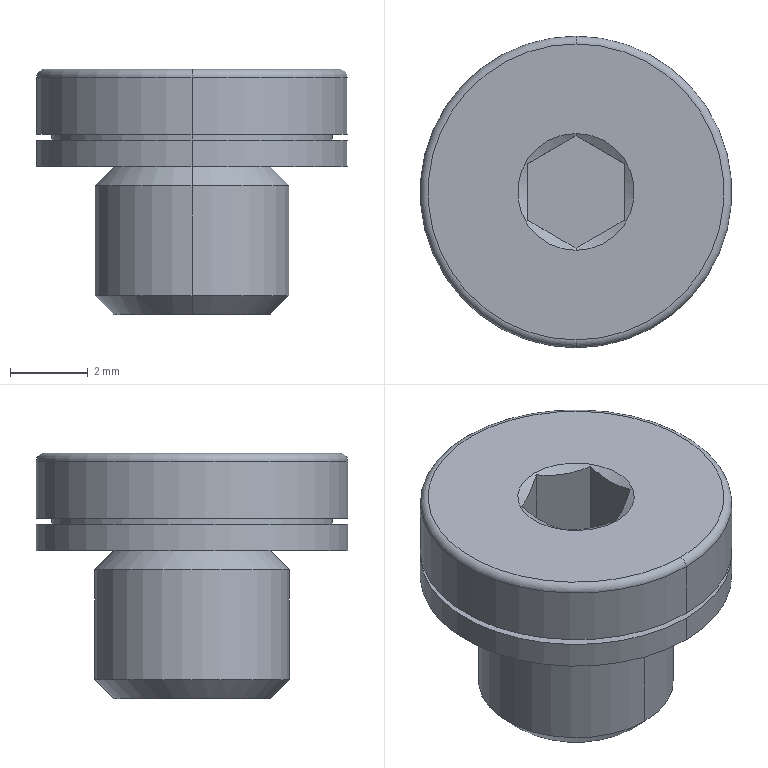Part | SolidWorks | features RefAxis 6, 3DProfileFeature 2, ICE 1, Revolution 1 | 1 solid | 28 faces | box 8 x 8 x 6.3 mm | volume 181.471 mm3 | plane 12 | cylinder 8 | cone 6 | torus 2 | commonest cylinder face diameters 8 x4 5 x2 7.2 x2
STEP:
#1=CARTESIAN_POINT('',(0.,-2.01,-3.8));
#2=VERTEX_POINT('',#1);
#3=CARTESIAN_POINT('',(0.,2.01,-3.8));
#4=VERTEX_POINT('',#3);
#5=CARTESIAN_POINT('',(0.,0.,-3.8));
#6=DIRECTION('',(0.,0.,1.));
#7=DIRECTION('',(0.,-1.,0.));
#8=AXIS2_PLACEMENT_3D('',#5,#6,#7);
#9=CIRCLE('',#8,2.01);
#10=EDGE_CURVE('',#2,#4,#9,.T.);
#11=ORIENTED_EDGE('',*,*,#10,.T.);
#12=CARTESIAN_POINT('',(0.,2.5,-3.309));
#13=VERTEX_POINT('',#12);
#14=CARTESIAN_POINT('',(0.,2.01,-3.8));
#15=DIRECTION('',(0.,0.7071,0.7071));
#16=VECTOR('',#15,1000.);
#17=LINE('',#14,#16);
#18=EDGE_CURVE('',#4,#13,#17,.T.);
#19=ORIENTED_EDGE('',*,*,#18,.T.);
#20=CARTESIAN_POINT('',(0.,-2.5,-3.309));
#21=VERTEX_POINT('',#20);
#22=CARTESIAN_POINT('',(0.,0.,-3.309));
#23=DIRECTION('',(0.,0.,1.));
#24=DIRECTION('',(0.,-1.,0.));
#25=AXIS2_PLACEMENT_3D('',#22,#23,#24);
#26=CIRCLE('',#25,2.5);
#27=EDGE_CURVE('',#21,#13,#26,.T.);
#28=ORIENTED_EDGE('',*,*,#27,.F.);
#29=CARTESIAN_POINT('',(0.,-2.01,-3.8));
#30=DIRECTION('',(0.,-0.7071,0.7071));
#31=VECTOR('',#30,1000.);
#32=LINE('',#29,#31);
#33=EDGE_CURVE('',#2,#21,#32,.T.);
#34=ORIENTED_EDGE('',*,*,#33,.F.);
#35=EDGE_LOOP('',(#11,#19,#28,#34));
#36=FACE_OUTER_BOUND('',#35,.T.);
#37=CARTESIAN_POINT('',(0.,0.,-3.8));
#38=DIRECTION('',(0.,0.,1.));
#39=DIRECTION('',(0.,-1.,0.));
#40=AXIS2_PLACEMENT_3D('',#37,#38,#39);
#41=CONICAL_SURFACE('',#40,2.01,0.7854);
#42=ADVANCED_FACE('',(#36),#41,.T.);
#43=ORIENTED_EDGE('',*,*,#27,.T.);
#44=CARTESIAN_POINT('',(0.,2.5,-0.4905));
#45=VERTEX_POINT('',#44);
#46=CARTESIAN_POINT('',(0.,2.5,-3.8));
#47=DIRECTION('',(0.,0.,1.));
#48=VECTOR('',#47,1000.);
#49=LINE('',#46,#48);
#50=EDGE_CURVE('',#13,#45,#49,.T.);
#51=ORIENTED_EDGE('',*,*,#50,.T.);
#52=CARTESIAN_POINT('',(0.,-2.5,-0.4905));
#53=VERTEX_POINT('',#52);
#54=CARTESIAN_POINT('',(0.,0.,-0.4905));
#55=DIRECTION('',(0.,0.,1.));
#56=DIRECTION('',(0.,-1.,0.));
#57=AXIS2_PLACEMENT_3D('',#54,#55,#56);
#58=CIRCLE('',#57,2.5);
#59=EDGE_CURVE('',#53,#45,#58,.T.);
#60=ORIENTED_EDGE('',*,*,#59,.F.);
#61=CARTESIAN_POINT('',(0.,-2.5,-3.8));
#62=DIRECTION('',(0.,0.,1.));
#63=VECTOR('',#62,1000.);
#64=LINE('',#61,#63);
#65=EDGE_CURVE('',#21,#53,#64,.T.);
#66=ORIENTED_EDGE('',*,*,#65,.F.);
#67=EDGE_LOOP('',(#43,#51,#60,#66));
#68=FACE_OUTER_BOUND('',#67,.T.);
#69=CARTESIAN_POINT('',(0.,0.,-3.8));
#70=DIRECTION('',(0.,0.,1.));
#71=DIRECTION('',(0.,-1.,0.));
#72=AXIS2_PLACEMENT_3D('',#69,#70,#71);
#73=CYLINDRICAL_SURFACE('',#72,2.5);
#74=ADVANCED_FACE('',(#68),#73,.T.);
#75=CARTESIAN_POINT('',(0.,-2.01,0.));
#76=VERTEX_POINT('',#75);
#77=CARTESIAN_POINT('',(0.,2.01,0.));
#78=VERTEX_POINT('',#77);
#79=CARTESIAN_POINT('',(0.,0.,0.));
#80=DIRECTION('',(0.,0.,1.));
#81=DIRECTION('',(0.,-1.,0.));
#82=AXIS2_PLACEMENT_3D('',#79,#80,#81);
#83=CIRCLE('',#82,2.01);
#84=EDGE_CURVE('',#76,#78,#83,.T.);
#85=ORIENTED_EDGE('',*,*,#84,.F.);
#86=CARTESIAN_POINT('',(0.,-2.5,-0.4905));
#87=DIRECTION('',(0.,-0.7071,-0.7071));
#88=VECTOR('',#87,1000.);
#89=LINE('',#86,#88);
#90=EDGE_CURVE('',#76,#53,#89,.T.);
#91=ORIENTED_EDGE('',*,*,#90,.T.);
#92=ORIENTED_EDGE('',*,*,#59,.T.);
#93=CARTESIAN_POINT('',(0.,2.5,-0.4905));
#94=DIRECTION('',(0.,0.7071,-0.7071));
#95=VECTOR('',#94,1000.);
#96=LINE('',#93,#95);
#97=EDGE_CURVE('',#78,#45,#96,.T.);
#98=ORIENTED_EDGE('',*,*,#97,.F.);
#99=EDGE_LOOP('',(#85,#91,#92,#98));
#100=FACE_OUTER_BOUND('',#99,.T.);
#101=CARTESIAN_POINT('',(0.,0.,-0.4905));
#102=DIRECTION('',(0.,0.,-1.));
#103=DIRECTION('',(0.,1.,0.));
#104=AXIS2_PLACEMENT_3D('',#101,#102,#103);
#105=CONICAL_SURFACE('',#104,2.5,0.7854);
#106=ADVANCED_FACE('',(#100),#105,.T.);
#107=CARTESIAN_POINT('',(0.,-4.,0.));
#108=VERTEX_POINT('',#107);
#109=CARTESIAN_POINT('',(0.,4.,0.));
#110=VERTEX_POINT('',#109);
#111=CARTESIAN_POINT('',(0.,0.,0.));
#112=DIRECTION('',(0.,0.,1.));
#113=DIRECTION('',(0.,-1.,0.));
#114=AXIS2_PLACEMENT_3D('',#111,#112,#113);
#115=CIRCLE('',#114,4.);
#116=EDGE_CURVE('',#108,#110,#115,.T.);
#117=ORIENTED_EDGE('',*,*,#116,.T.);
#118=CARTESIAN_POINT('',(0.,4.,0.6833));
#119=VERTEX_POINT('',#118);
#120=CARTESIAN_POINT('',(0.,4.,-3.8));
#121=DIRECTION('',(0.,0.,1.));
#122=VECTOR('',#121,1000.);
#123=LINE('',#120,#122);
#124=EDGE_CURVE('',#110,#119,#123,.T.);
#125=ORIENTED_EDGE('',*,*,#124,.T.);
#126=CARTESIAN_POINT('',(0.,-4.,0.6833));
#127=VERTEX_POINT('',#126);
#128=CARTESIAN_POINT('',(0.,0.,0.6833));
#129=DIRECTION('',(0.,0.,1.));
#130=DIRECTION('',(0.,-1.,0.));
#131=AXIS2_PLACEMENT_3D('',#128,#129,#130);
#132=CIRCLE('',#131,4.);
#133=EDGE_CURVE('',#127,#119,#132,.T.);
#134=ORIENTED_EDGE('',*,*,#133,.F.);
#135=CARTESIAN_POINT('',(0.,-4.,-3.8));
#136=DIRECTION('',(0.,0.,1.));
#137=VECTOR('',#136,1000.);
#138=LINE('',#135,#137);
#139=EDGE_CURVE('',#108,#127,#138,.T.);
#140=ORIENTED_EDGE('',*,*,#139,.F.);
#141=EDGE_LOOP('',(#117,#125,#134,#140));
#142=FACE_OUTER_BOUND('',#141,.T.);
#143=CARTESIAN_POINT('',(0.,0.,-3.8));
#144=DIRECTION('',(0.,0.,1.));
#145=DIRECTION('',(0.,-1.,0.));
#146=AXIS2_PLACEMENT_3D('',#143,#144,#145);
#147=CYLINDRICAL_SURFACE('',#146,4.);
#148=ADVANCED_FACE('',(#142),#147,.T.);
#149=CARTESIAN_POINT('',(0.,-3.6,0.6833));
#150=VERTEX_POINT('',#149);
#151=CARTESIAN_POINT('',(0.,3.6,0.6833));
#152=VERTEX_POINT('',#151);
#153=CARTESIAN_POINT('',(0.,0.,0.6833));
#154=DIRECTION('',(0.,0.,1.));
#155=DIRECTION('',(0.,-1.,0.));
#156=AXIS2_PLACEMENT_3D('',#153,#154,#155);
#157=CIRCLE('',#156,3.6);
#158=EDGE_CURVE('',#150,#152,#157,.T.);
#159=ORIENTED_EDGE('',*,*,#158,.T.);
#160=CARTESIAN_POINT('',(0.,3.6,0.8333));
#161=VERTEX_POINT('',#160);
#162=CARTESIAN_POINT('',(0.,3.6,-3.8));
#163=DIRECTION('',(0.,0.,1.));
#164=VECTOR('',#163,1000.);
#165=LINE('',#162,#164);
#166=EDGE_CURVE('',#152,#161,#165,.T.);
#167=ORIENTED_EDGE('',*,*,#166,.T.);
#168=CARTESIAN_POINT('',(0.,-3.6,0.8333));
#169=VERTEX_POINT('',#168);
#170=CARTESIAN_POINT('',(0.,0.,0.8333));
#171=DIRECTION('',(0.,0.,1.));
#172=DIRECTION('',(0.,-1.,0.));
#173=AXIS2_PLACEMENT_3D('',#170,#171,#172);
#174=CIRCLE('',#173,3.6);
#175=EDGE_CURVE('',#169,#161,#174,.T.);
#176=ORIENTED_EDGE('',*,*,#175,.F.);
#177=CARTESIAN_POINT('',(0.,-3.6,-3.8));
#178=DIRECTION('',(0.,0.,1.));
#179=VECTOR('',#178,1000.);
#180=LINE('',#177,#179);
#181=EDGE_CURVE('',#150,#169,#180,.T.);
#182=ORIENTED_EDGE('',*,*,#181,.F.);
#183=EDGE_LOOP('',(#159,#167,#176,#182));
#184=FACE_OUTER_BOUND('',#183,.T.);
#185=CARTESIAN_POINT('',(0.,0.,-3.8));
#186=DIRECTION('',(0.,0.,1.));
#187=DIRECTION('',(0.,-1.,0.));
#188=AXIS2_PLACEMENT_3D('',#185,#186,#187);
#189=CYLINDRICAL_SURFACE('',#188,3.6);
#190=ADVANCED_FACE('',(#184),#189,.T.);
#191=CARTESIAN_POINT('',(0.,-4.,0.8333));
#192=VERTEX_POINT('',#191);
#193=CARTESIAN_POINT('',(0.,4.,0.8333));
#194=VERTEX_POINT('',#193);
#195=CARTESIAN_POINT('',(0.,0.,0.8333));
#196=DIRECTION('',(0.,0.,1.));
#197=DIRECTION('',(0.,-1.,0.));
#198=AXIS2_PLACEMENT_3D('',#195,#196,#197);
#199=CIRCLE('',#198,4.);
#200=EDGE_CURVE('',#192,#194,#199,.T.);
#201=ORIENTED_EDGE('',*,*,#200,.T.);
#202=CARTESIAN_POINT('',(0.,4.,2.3));
#203=VERTEX_POINT('',#202);
#204=CARTESIAN_POINT('',(0.,4.,-3.8));
#205=DIRECTION('',(0.,0.,1.));
#206=VECTOR('',#205,1000.);
#207=LINE('',#204,#206);
#208=EDGE_CURVE('',#194,#203,#207,.T.);
#209=ORIENTED_EDGE('',*,*,#208,.T.);
#210=CARTESIAN_POINT('',(0.,-4.,2.3));
#211=VERTEX_POINT('',#210);
#212=CARTESIAN_POINT('',(0.,0.,2.3));
#213=DIRECTION('',(0.,0.,1.));
#214=DIRECTION('',(0.,-1.,0.));
#215=AXIS2_PLACEMENT_3D('',#212,#213,#214);
#216=CIRCLE('',#215,4.);
#217=EDGE_CURVE('',#211,#203,#216,.T.);
#218=ORIENTED_EDGE('',*,*,#217,.F.);
#219=CARTESIAN_POINT('',(0.,-4.,-3.8));
#220=DIRECTION('',(0.,0.,1.));
#221=VECTOR('',#220,1000.);
#222=LINE('',#219,#221);
#223=EDGE_CURVE('',#192,#211,#222,.T.);
#224=ORIENTED_EDGE('',*,*,#223,.F.);
#225=EDGE_LOOP('',(#201,#209,#218,#224));
#226=FACE_OUTER_BOUND('',#225,.T.);
#227=CARTESIAN_POINT('',(0.,0.,-3.8));
#228=DIRECTION('',(0.,0.,1.));
#229=DIRECTION('',(0.,-1.,0.));
#230=AXIS2_PLACEMENT_3D('',#227,#228,#229);
#231=CYLINDRICAL_SURFACE('',#230,4.);
#232=ADVANCED_FACE('',(#226),#231,.T.);
#233=ORIENTED_EDGE('',*,*,#217,.T.);
#234=CARTESIAN_POINT('',(0.,3.8,2.5));
#235=VERTEX_POINT('',#234);
#236=CARTESIAN_POINT('',(0.,3.8,2.3));
#237=DIRECTION('',(1.,0.,0.));
#238=DIRECTION('',(0.,1.,0.));
#239=AXIS2_PLACEMENT_3D('',#236,#237,#238);
#240=CIRCLE('',#239,0.2);
#241=EDGE_CURVE('',#203,#235,#240,.T.);
#242=ORIENTED_EDGE('',*,*,#241,.T.);
#243=CARTESIAN_POINT('',(0.,-3.8,2.5));
#244=VERTEX_POINT('',#243);
#245=CARTESIAN_POINT('',(0.,0.,2.5));
#246=DIRECTION('',(0.,0.,1.));
#247=DIRECTION('',(0.,-1.,0.));
#248=AXIS2_PLACEMENT_3D('',#245,#246,#247);
#249=CIRCLE('',#248,3.8);
#250=EDGE_CURVE('',#244,#235,#249,.T.);
#251=ORIENTED_EDGE('',*,*,#250,.F.);
#252=CARTESIAN_POINT('',(0.,-3.8,2.3));
#253=DIRECTION('',(-1.,0.,0.));
#254=DIRECTION('',(0.,0.,1.));
#255=AXIS2_PLACEMENT_3D('',#252,#253,#254);
#256=CIRCLE('',#255,0.2);
#257=EDGE_CURVE('',#211,#244,#256,.T.);
#258=ORIENTED_EDGE('',*,*,#257,.F.);
#259=EDGE_LOOP('',(#233,#242,#251,#258));
#260=FACE_OUTER_BOUND('',#259,.T.);
#261=CARTESIAN_POINT('',(0.,0.,2.3));
#262=DIRECTION('',(0.,0.,1.));
#263=DIRECTION('',(0.,-1.,0.));
#264=AXIS2_PLACEMENT_3D('',#261,#262,#263);
#265=TOROIDAL_SURFACE('',#264,3.8,0.2);
#266=ADVANCED_FACE('',(#260),#265,.T.);
#267=CARTESIAN_POINT('',(-1.25,0.7217,2.467));
#268=VERTEX_POINT('',#267);
#269=CARTESIAN_POINT('',(0.,1.443,2.467));
#270=VERTEX_POINT('',#269);
#271=CARTESIAN_POINT('',(-1.25,0.7217,2.467));
#272=CARTESIAN_POINT('',(-1.046,0.8395,2.399));
#273=CARTESIAN_POINT('',(-0.8387,0.9591,2.356));
#274=CARTESIAN_POINT('',(-0.4136,1.205,2.356));
#275=CARTESIAN_POINT('',(-0.2044,1.325,2.399));
#276=CARTESIAN_POINT('',(0.,1.443,2.467));
#277=B_SPLINE_CURVE_WITH_KNOTS('',3,(#271,#272,#273,#274,#275,#276),.UNSPECIFIED.,.F.,.F.,(4,2,4),(0.000000238,0.0007291,0.001458),.UNSPECIFIED.);
#278=EDGE_CURVE('',#268,#270,#277,.T.);
#279=ORIENTED_EDGE('',*,*,#278,.T.);
#280=CARTESIAN_POINT('',(0.,1.5,2.5));
#281=VERTEX_POINT('',#280);
#282=CARTESIAN_POINT('',(0.,1.5,2.5));
#283=DIRECTION('',(0.,0.866,0.5));
#284=VECTOR('',#283,1000.);
#285=LINE('',#282,#284);
#286=EDGE_CURVE('',#270,#281,#285,.T.);
#287=ORIENTED_EDGE('',*,*,#286,.T.);
#288=CARTESIAN_POINT('',(0.,-1.5,2.5));
#289=VERTEX_POINT('',#288);
#290=CARTESIAN_POINT('',(0.,0.,2.5));
#291=DIRECTION('',(0.,0.,1.));
#292=DIRECTION('',(0.,-1.,0.));
#293=AXIS2_PLACEMENT_3D('',#290,#291,#292);
#294=CIRCLE('',#293,1.5);
#295=EDGE_CURVE('',#281,#289,#294,.T.);
#296=ORIENTED_EDGE('',*,*,#295,.T.);
#297=CARTESIAN_POINT('',(0.,-1.443,2.467));
#298=VERTEX_POINT('',#297);
#299=CARTESIAN_POINT('',(0.,-1.5,2.5));
#300=DIRECTION('',(0.,-0.866,0.5));
#301=VECTOR('',#300,1000.);
#302=LINE('',#299,#301);
#303=EDGE_CURVE('',#298,#289,#302,.T.);
#304=ORIENTED_EDGE('',*,*,#303,.F.);
#305=CARTESIAN_POINT('',(-1.25,-0.7217,2.467));
#306=VERTEX_POINT('',#305);
#307=CARTESIAN_POINT('',(0.,-1.443,2.467));
#308=CARTESIAN_POINT('',(-0.2041,-1.326,2.399));
#309=CARTESIAN_POINT('',(-0.4113,-1.206,2.356));
#310=CARTESIAN_POINT('',(-0.8364,-0.9605,2.356));
#311=CARTESIAN_POINT('',(-1.046,-0.8397,2.399));
#312=CARTESIAN_POINT('',(-1.25,-0.7217,2.467));
#313=B_SPLINE_CURVE_WITH_KNOTS('',3,(#307,#308,#309,#310,#311,#312),.UNSPECIFIED.,.F.,.F.,(4,2,4),(0.000000238,0.0007291,0.001458),.UNSPECIFIED.);
#314=EDGE_CURVE('',#298,#306,#313,.T.);
#315=ORIENTED_EDGE('',*,*,#314,.T.);
#316=CARTESIAN_POINT('',(-1.25,-0.7217,2.467));
#317=CARTESIAN_POINT('',(-1.25,-0.4871,2.4));
#318=CARTESIAN_POINT('',(-1.25,-0.2436,2.356));
#319=CARTESIAN_POINT('',(-1.25,0.1221,2.356));
#320=CARTESIAN_POINT('',(-1.25,0.2456,2.366));
#321=CARTESIAN_POINT('',(-1.25,0.4868,2.406));
#322=CARTESIAN_POINT('',(-1.25,0.605,2.434));
#323=CARTESIAN_POINT('',(-1.25,0.7217,2.467));
#324=B_SPLINE_CURVE_WITH_KNOTS('',3,(#316,#317,#318,#319,#320,#321,#322,#323),.UNSPECIFIED.,.F.,.F.,(4,2,2,4),(0.001248,0.001978,0.002343,0.002708),.UNSPECIFIED.);
#325=EDGE_CURVE('',#306,#268,#324,.T.);
#326=ORIENTED_EDGE('',*,*,#325,.T.);
#327=EDGE_LOOP('',(#279,#287,#296,#304,#315,#326));
#328=FACE_OUTER_BOUND('',#327,.T.);
#329=CARTESIAN_POINT('',(0.,0.,2.5));
#330=DIRECTION('',(0.,0.,1.));
#331=DIRECTION('',(0.,-1.,0.));
#332=AXIS2_PLACEMENT_3D('',#329,#330,#331);
#333=CONICAL_SURFACE('',#332,1.5,1.047);
#334=ADVANCED_FACE('',(#328),#333,.F.);
#335=ORIENTED_EDGE('',*,*,#286,.F.);
#336=CARTESIAN_POINT('',(1.25,0.7217,2.467));
#337=VERTEX_POINT('',#336);
#338=CARTESIAN_POINT('',(0.,1.443,2.467));
#339=CARTESIAN_POINT('',(0.2041,1.326,2.399));
#340=CARTESIAN_POINT('',(0.4113,1.206,2.356));
#341=CARTESIAN_POINT('',(0.8364,0.9605,2.356));
#342=CARTESIAN_POINT('',(1.046,0.8397,2.399));
#343=CARTESIAN_POINT('',(1.25,0.7217,2.467));
#344=B_SPLINE_CURVE_WITH_KNOTS('',3,(#338,#339,#340,#341,#342,#343),.UNSPECIFIED.,.F.,.F.,(4,2,4),(0.000000238,0.0007291,0.001458),.UNSPECIFIED.);
#345=EDGE_CURVE('',#270,#337,#344,.T.);
#346=ORIENTED_EDGE('',*,*,#345,.T.);
#347=CARTESIAN_POINT('',(1.25,-0.7217,2.467));
#348=VERTEX_POINT('',#347);
#349=CARTESIAN_POINT('',(1.25,0.7217,2.467));
#350=CARTESIAN_POINT('',(1.25,0.605,2.434));
#351=CARTESIAN_POINT('',(1.25,0.4868,2.406));
#352=CARTESIAN_POINT('',(1.25,0.2456,2.366));
#353=CARTESIAN_POINT('',(1.25,0.1221,2.356));
#354=CARTESIAN_POINT('',(1.25,-0.2436,2.356));
#355=CARTESIAN_POINT('',(1.25,-0.4871,2.4));
#356=CARTESIAN_POINT('',(1.25,-0.7217,2.467));
#357=B_SPLINE_CURVE_WITH_KNOTS('',3,(#349,#350,#351,#352,#353,#354,#355,#356),.UNSPECIFIED.,.F.,.F.,(4,2,2,4),(0.003877,0.004242,0.004608,0.005339),.UNSPECIFIED.);
#358=EDGE_CURVE('',#337,#348,#357,.T.);
#359=ORIENTED_EDGE('',*,*,#358,.T.);
#360=CARTESIAN_POINT('',(1.25,-0.7217,2.467));
#361=CARTESIAN_POINT('',(1.046,-0.8395,2.399));
#362=CARTESIAN_POINT('',(0.8387,-0.9591,2.356));
#363=CARTESIAN_POINT('',(0.4136,-1.205,2.356));
#364=CARTESIAN_POINT('',(0.2044,-1.325,2.399));
#365=CARTESIAN_POINT('',(0.,-1.443,2.467));
#366=B_SPLINE_CURVE_WITH_KNOTS('',3,(#360,#361,#362,#363,#364,#365),.UNSPECIFIED.,.F.,.F.,(4,2,4),(0.000000238,0.0007291,0.001458),.UNSPECIFIED.);
#367=EDGE_CURVE('',#348,#298,#366,.T.);
#368=ORIENTED_EDGE('',*,*,#367,.T.);
#369=ORIENTED_EDGE('',*,*,#303,.T.);
#370=CARTESIAN_POINT('',(0.,0.,2.5));
#371=DIRECTION('',(0.,0.,1.));
#372=DIRECTION('',(0.,-1.,0.));
#373=AXIS2_PLACEMENT_3D('',#370,#371,#372);
#374=CIRCLE('',#373,1.5);
#375=EDGE_CURVE('',#289,#281,#374,.T.);
#376=ORIENTED_EDGE('',*,*,#375,.T.);
#377=EDGE_LOOP('',(#335,#346,#359,#368,#369,#376));
#378=FACE_OUTER_BOUND('',#377,.T.);
#379=CARTESIAN_POINT('',(0.,0.,2.5));
#380=DIRECTION('',(0.,0.,1.));
#381=DIRECTION('',(0.,-1.,0.));
#382=AXIS2_PLACEMENT_3D('',#379,#380,#381);
#383=CONICAL_SURFACE('',#382,1.5,1.047);
#384=ADVANCED_FACE('',(#378),#383,.F.);
#385=ORIENTED_EDGE('',*,*,#375,.F.);
#386=ORIENTED_EDGE('',*,*,#295,.F.);
#387=EDGE_LOOP('',(#385,#386));
#388=FACE_BOUND('',#387,.T.);
#389=ORIENTED_EDGE('',*,*,#250,.T.);
#390=CARTESIAN_POINT('',(0.,0.,2.5));
#391=DIRECTION('',(0.,0.,1.));
#392=DIRECTION('',(0.,-1.,0.));
#393=AXIS2_PLACEMENT_3D('',#390,#391,#392);
#394=CIRCLE('',#393,3.8);
#395=EDGE_CURVE('',#235,#244,#394,.T.);
#396=ORIENTED_EDGE('',*,*,#395,.T.);
#397=EDGE_LOOP('',(#389,#396));
#398=FACE_OUTER_BOUND('',#397,.T.);
#399=CARTESIAN_POINT('',(0.,1.5,2.5));
#400=DIRECTION('',(0.,0.,-1.));
#401=DIRECTION('',(0.,1.,0.));
#402=AXIS2_PLACEMENT_3D('',#399,#400,#401);
#403=PLANE('',#402);
#404=ADVANCED_FACE('',(#388,#398),#403,.F.);
#405=ORIENTED_EDGE('',*,*,#241,.F.);
#406=CARTESIAN_POINT('',(0.,0.,2.3));
#407=DIRECTION('',(0.,0.,1.));
#408=DIRECTION('',(0.,-1.,0.));
#409=AXIS2_PLACEMENT_3D('',#406,#407,#408);
#410=CIRCLE('',#409,4.);
#411=EDGE_CURVE('',#203,#211,#410,.T.);
#412=ORIENTED_EDGE('',*,*,#411,.T.);
#413=ORIENTED_EDGE('',*,*,#257,.T.);
#414=ORIENTED_EDGE('',*,*,#395,.F.);
#415=EDGE_LOOP('',(#405,#412,#413,#414));
#416=FACE_OUTER_BOUND('',#415,.T.);
#417=CARTESIAN_POINT('',(0.,0.,2.3));
#418=DIRECTION('',(0.,0.,1.));
#419=DIRECTION('',(0.,-1.,0.));
#420=AXIS2_PLACEMENT_3D('',#417,#418,#419);
#421=TOROIDAL_SURFACE('',#420,3.8,0.2);
#422=ADVANCED_FACE('',(#416),#421,.T.);
#423=ORIENTED_EDGE('',*,*,#208,.F.);
#424=CARTESIAN_POINT('',(0.,0.,0.8333));
#425=DIRECTION('',(0.,0.,1.));
#426=DIRECTION('',(0.,-1.,0.));
#427=AXIS2_PLACEMENT_3D('',#424,#425,#426);
#428=CIRCLE('',#427,4.);
#429=EDGE_CURVE('',#194,#192,#428,.T.);
#430=ORIENTED_EDGE('',*,*,#429,.T.);
#431=ORIENTED_EDGE('',*,*,#223,.T.);
#432=ORIENTED_EDGE('',*,*,#411,.F.);
#433=EDGE_LOOP('',(#423,#430,#431,#432));
#434=FACE_OUTER_BOUND('',#433,.T.);
#435=CARTESIAN_POINT('',(0.,0.,-3.8));
#436=DIRECTION('',(0.,0.,1.));
#437=DIRECTION('',(0.,-1.,0.));
#438=AXIS2_PLACEMENT_3D('',#435,#436,#437);
#439=CYLINDRICAL_SURFACE('',#438,4.);
#440=ADVANCED_FACE('',(#434),#439,.T.);
#441=ORIENTED_EDGE('',*,*,#200,.F.);
#442=ORIENTED_EDGE('',*,*,#429,.F.);
#443=EDGE_LOOP('',(#441,#442));
#444=FACE_OUTER_BOUND('',#443,.T.);
#445=ORIENTED_EDGE('',*,*,#175,.T.);
#446=CARTESIAN_POINT('',(0.,0.,0.8333));
#447=DIRECTION('',(0.,0.,1.));
#448=DIRECTION('',(0.,-1.,0.));
#449=AXIS2_PLACEMENT_3D('',#446,#447,#448);
#450=CIRCLE('',#449,3.6);
#451=EDGE_CURVE('',#161,#169,#450,.T.);
#452=ORIENTED_EDGE('',*,*,#451,.T.);
#453=EDGE_LOOP('',(#445,#452));
#454=FACE_BOUND('',#453,.T.);
#455=CARTESIAN_POINT('',(0.,4.,0.8333));
#456=DIRECTION('',(0.,0.,1.));
#457=DIRECTION('',(0.,-1.,0.));
#458=AXIS2_PLACEMENT_3D('',#455,#456,#457);
#459=PLANE('',#458);
#460=ADVANCED_FACE('',(#444,#454),#459,.F.);
#461=ORIENTED_EDGE('',*,*,#166,.F.);
#462=CARTESIAN_POINT('',(0.,0.,0.6833));
#463=DIRECTION('',(0.,0.,1.));
#464=DIRECTION('',(0.,-1.,0.));
#465=AXIS2_PLACEMENT_3D('',#462,#463,#464);
#466=CIRCLE('',#465,3.6);
#467=EDGE_CURVE('',#152,#150,#466,.T.);
#468=ORIENTED_EDGE('',*,*,#467,.T.);
#469=ORIENTED_EDGE('',*,*,#181,.T.);
#470=ORIENTED_EDGE('',*,*,#451,.F.);
#471=EDGE_LOOP('',(#461,#468,#469,#470));
#472=FACE_OUTER_BOUND('',#471,.T.);
#473=CARTESIAN_POINT('',(0.,0.,-3.8));
#474=DIRECTION('',(0.,0.,1.));
#475=DIRECTION('',(0.,-1.,0.));
#476=AXIS2_PLACEMENT_3D('',#473,#474,#475);
#477=CYLINDRICAL_SURFACE('',#476,3.6);
#478=ADVANCED_FACE('',(#472),#477,.T.);
#479=ORIENTED_EDGE('',*,*,#158,.F.);
#480=ORIENTED_EDGE('',*,*,#467,.F.);
#481=EDGE_LOOP('',(#479,#480));
#482=FACE_BOUND('',#481,.T.);
#483=ORIENTED_EDGE('',*,*,#133,.T.);
#484=CARTESIAN_POINT('',(0.,0.,0.6833));
#485=DIRECTION('',(0.,0.,1.));
#486=DIRECTION('',(0.,-1.,0.));
#487=AXIS2_PLACEMENT_3D('',#484,#485,#486);
#488=CIRCLE('',#487,4.);
#489=EDGE_CURVE('',#119,#127,#488,.T.);
#490=ORIENTED_EDGE('',*,*,#489,.T.);
#491=EDGE_LOOP('',(#483,#490));
#492=FACE_OUTER_BOUND('',#491,.T.);
#493=CARTESIAN_POINT('',(0.,3.6,0.6833));
#494=DIRECTION('',(0.,0.,-1.));
#495=DIRECTION('',(0.,1.,0.));
#496=AXIS2_PLACEMENT_3D('',#493,#494,#495);
#497=PLANE('',#496);
#498=ADVANCED_FACE('',(#482,#492),#497,.F.);
#499=ORIENTED_EDGE('',*,*,#124,.F.);
#500=CARTESIAN_POINT('',(0.,0.,0.));
#501=DIRECTION('',(0.,0.,1.));
#502=DIRECTION('',(0.,-1.,0.));
#503=AXIS2_PLACEMENT_3D('',#500,#501,#502);
#504=CIRCLE('',#503,4.);
#505=EDGE_CURVE('',#110,#108,#504,.T.);
#506=ORIENTED_EDGE('',*,*,#505,.T.);
#507=ORIENTED_EDGE('',*,*,#139,.T.);
#508=ORIENTED_EDGE('',*,*,#489,.F.);
#509=EDGE_LOOP('',(#499,#506,#507,#508));
#510=FACE_OUTER_BOUND('',#509,.T.);
#511=CARTESIAN_POINT('',(0.,0.,-3.8));
#512=DIRECTION('',(0.,0.,1.));
#513=DIRECTION('',(0.,-1.,0.));
#514=AXIS2_PLACEMENT_3D('',#511,#512,#513);
#515=CYLINDRICAL_SURFACE('',#514,4.);
#516=ADVANCED_FACE('',(#510),#515,.T.);
#517=ORIENTED_EDGE('',*,*,#116,.F.);
#518=ORIENTED_EDGE('',*,*,#505,.F.);
#519=EDGE_LOOP('',(#517,#518));
#520=FACE_OUTER_BOUND('',#519,.T.);
#521=CARTESIAN_POINT('',(0.,0.,0.));
#522=DIRECTION('',(0.,0.,1.));
#523=DIRECTION('',(0.,-1.,0.));
#524=AXIS2_PLACEMENT_3D('',#521,#522,#523);
#525=CIRCLE('',#524,2.01);
#526=EDGE_CURVE('',#78,#76,#525,.T.);
#527=ORIENTED_EDGE('',*,*,#526,.T.);
#528=ORIENTED_EDGE('',*,*,#84,.T.);
#529=EDGE_LOOP('',(#527,#528));
#530=FACE_BOUND('',#529,.T.);
#531=CARTESIAN_POINT('',(0.,4.,0.));
#532=DIRECTION('',(0.,0.,1.));
#533=DIRECTION('',(0.,-1.,0.));
#534=AXIS2_PLACEMENT_3D('',#531,#532,#533);
#535=PLANE('',#534);
#536=ADVANCED_FACE('',(#520,#530),#535,.F.);
#537=ORIENTED_EDGE('',*,*,#90,.F.);
#538=ORIENTED_EDGE('',*,*,#526,.F.);
#539=ORIENTED_EDGE('',*,*,#97,.T.);
#540=CARTESIAN_POINT('',(0.,0.,-0.4905));
#541=DIRECTION('',(0.,0.,1.));
#542=DIRECTION('',(0.,-1.,0.));
#543=AXIS2_PLACEMENT_3D('',#540,#541,#542);
#544=CIRCLE('',#543,2.5);
#545=EDGE_CURVE('',#45,#53,#544,.T.);
#546=ORIENTED_EDGE('',*,*,#545,.T.);
#547=EDGE_LOOP('',(#537,#538,#539,#546));
#548=FACE_OUTER_BOUND('',#547,.T.);
#549=CARTESIAN_POINT('',(0.,0.,-0.4905));
#550=DIRECTION('',(0.,0.,-1.));
#551=DIRECTION('',(0.,1.,0.));
#552=AXIS2_PLACEMENT_3D('',#549,#550,#551);
#553=CONICAL_SURFACE('',#552,2.5,0.7854);
#554=ADVANCED_FACE('',(#548),#553,.T.);
#555=ORIENTED_EDGE('',*,*,#50,.F.);
#556=CARTESIAN_POINT('',(0.,0.,-3.309));
#557=DIRECTION('',(0.,0.,1.));
#558=DIRECTION('',(0.,-1.,0.));
#559=AXIS2_PLACEMENT_3D('',#556,#557,#558);
#560=CIRCLE('',#559,2.5);
#561=EDGE_CURVE('',#13,#21,#560,.T.);
#562=ORIENTED_EDGE('',*,*,#561,.T.);
#563=ORIENTED_EDGE('',*,*,#65,.T.);
#564=ORIENTED_EDGE('',*,*,#545,.F.);
#565=EDGE_LOOP('',(#555,#562,#563,#564));
#566=FACE_OUTER_BOUND('',#565,.T.);
#567=CARTESIAN_POINT('',(0.,0.,-3.8));
#568=DIRECTION('',(0.,0.,1.));
#569=DIRECTION('',(0.,-1.,0.));
#570=AXIS2_PLACEMENT_3D('',#567,#568,#569);
#571=CYLINDRICAL_SURFACE('',#570,2.5);
#572=ADVANCED_FACE('',(#566),#571,.T.);
#573=ORIENTED_EDGE('',*,*,#18,.F.);
#574=CARTESIAN_POINT('',(0.,0.,-3.8));
#575=DIRECTION('',(0.,0.,1.));
#576=DIRECTION('',(0.,-1.,0.));
#577=AXIS2_PLACEMENT_3D('',#574,#575,#576);
#578=CIRCLE('',#577,2.01);
#579=EDGE_CURVE('',#4,#2,#578,.T.);
#580=ORIENTED_EDGE('',*,*,#579,.T.);
#581=ORIENTED_EDGE('',*,*,#33,.T.);
#582=ORIENTED_EDGE('',*,*,#561,.F.);
#583=EDGE_LOOP('',(#573,#580,#581,#582));
#584=FACE_OUTER_BOUND('',#583,.T.);
#585=CARTESIAN_POINT('',(0.,0.,-3.8));
#586=DIRECTION('',(0.,0.,1.));
#587=DIRECTION('',(0.,-1.,0.));
#588=AXIS2_PLACEMENT_3D('',#585,#586,#587);
#589=CONICAL_SURFACE('',#588,2.01,0.7854);
#590=ADVANCED_FACE('',(#584),#589,.T.);
#591=ORIENTED_EDGE('',*,*,#10,.F.);
#592=ORIENTED_EDGE('',*,*,#579,.F.);
#593=EDGE_LOOP('',(#591,#592));
#594=FACE_OUTER_BOUND('',#593,.T.);
#595=CARTESIAN_POINT('',(0.,2.01,-3.8));
#596=DIRECTION('',(0.,0.,1.));
#597=DIRECTION('',(0.,-1.,0.));
#598=AXIS2_PLACEMENT_3D('',#595,#596,#597);
#599=PLANE('',#598);
#600=ADVANCED_FACE('',(#594),#599,.F.);
#601=CARTESIAN_POINT('',(-1.25,-0.7217,0.));
#602=VERTEX_POINT('',#601);
#603=CARTESIAN_POINT('',(-1.25,-0.7217,0.));
#604=DIRECTION('',(0.,0.,1.));
#605=VECTOR('',#604,1000.);
#606=LINE('',#603,#605);
#607=EDGE_CURVE('',#602,#306,#606,.T.);
#608=ORIENTED_EDGE('',*,*,#607,.F.);
#609=CARTESIAN_POINT('',(-1.25,0.7217,0.));
#610=VERTEX_POINT('',#609);
#611=CARTESIAN_POINT('',(-1.25,0.7217,0.));
#612=DIRECTION('',(0.,-1.,0.));
#613=VECTOR('',#612,1000.);
#614=LINE('',#611,#613);
#615=EDGE_CURVE('',#610,#602,#614,.T.);
#616=ORIENTED_EDGE('',*,*,#615,.F.);
#617=CARTESIAN_POINT('',(-1.25,0.7217,0.));
#618=DIRECTION('',(0.,0.,1.));
#619=VECTOR('',#618,1000.);
#620=LINE('',#617,#619);
#621=EDGE_CURVE('',#610,#268,#620,.T.);
#622=ORIENTED_EDGE('',*,*,#621,.T.);
#623=ORIENTED_EDGE('',*,*,#325,.F.);
#624=EDGE_LOOP('',(#608,#616,#622,#623));
#625=FACE_OUTER_BOUND('',#624,.T.);
#626=CARTESIAN_POINT('',(-1.25,0.7217,0.));
#627=DIRECTION('',(-1.,0.,0.));
#628=DIRECTION('',(0.,0.,1.));
#629=AXIS2_PLACEMENT_3D('',#626,#627,#628);
#630=PLANE('',#629);
#631=ADVANCED_FACE('',(#625),#630,.F.);
#632=ORIENTED_EDGE('',*,*,#621,.F.);
#633=CARTESIAN_POINT('',(0.,1.443,0.));
#634=VERTEX_POINT('',#633);
#635=CARTESIAN_POINT('',(0.,1.443,0.));
#636=DIRECTION('',(-0.866,-0.5,0.));
#637=VECTOR('',#636,1000.);
#638=LINE('',#635,#637);
#639=EDGE_CURVE('',#634,#610,#638,.T.);
#640=ORIENTED_EDGE('',*,*,#639,.F.);
#641=CARTESIAN_POINT('',(0.,1.443,0.));
#642=DIRECTION('',(0.,0.,1.));
#643=VECTOR('',#642,1000.);
#644=LINE('',#641,#643);
#645=EDGE_CURVE('',#634,#270,#644,.T.);
#646=ORIENTED_EDGE('',*,*,#645,.T.);
#647=ORIENTED_EDGE('',*,*,#278,.F.);
#648=EDGE_LOOP('',(#632,#640,#646,#647));
#649=FACE_OUTER_BOUND('',#648,.T.);
#650=CARTESIAN_POINT('',(0.,1.443,0.));
#651=DIRECTION('',(-0.5,0.866,0.));
#652=DIRECTION('',(-0.866,-0.5,0.));
#653=AXIS2_PLACEMENT_3D('',#650,#651,#652);
#654=PLANE('',#653);
#655=ADVANCED_FACE('',(#649),#654,.F.);
#656=ORIENTED_EDGE('',*,*,#645,.F.);
#657=CARTESIAN_POINT('',(1.25,0.7217,0.));
#658=VERTEX_POINT('',#657);
#659=CARTESIAN_POINT('',(1.25,0.7217,0.));
#660=DIRECTION('',(-0.866,0.5,0.));
#661=VECTOR('',#660,1000.);
#662=LINE('',#659,#661);
#663=EDGE_CURVE('',#658,#634,#662,.T.);
#664=ORIENTED_EDGE('',*,*,#663,.F.);
#665=CARTESIAN_POINT('',(1.25,0.7217,0.));
#666=DIRECTION('',(0.,0.,1.));
#667=VECTOR('',#666,1000.);
#668=LINE('',#665,#667);
#669=EDGE_CURVE('',#658,#337,#668,.T.);
#670=ORIENTED_EDGE('',*,*,#669,.T.);
#671=ORIENTED_EDGE('',*,*,#345,.F.);
#672=EDGE_LOOP('',(#656,#664,#670,#671));
#673=FACE_OUTER_BOUND('',#672,.T.);
#674=CARTESIAN_POINT('',(1.25,0.7217,0.));
#675=DIRECTION('',(0.5,0.866,0.));
#676=DIRECTION('',(-0.866,0.5,0.));
#677=AXIS2_PLACEMENT_3D('',#674,#675,#676);
#678=PLANE('',#677);
#679=ADVANCED_FACE('',(#673),#678,.F.);
#680=ORIENTED_EDGE('',*,*,#669,.F.);
#681=CARTESIAN_POINT('',(1.25,-0.7217,0.));
#682=VERTEX_POINT('',#681);
#683=CARTESIAN_POINT('',(1.25,-0.7217,0.));
#684=DIRECTION('',(0.,1.,0.));
#685=VECTOR('',#684,1000.);
#686=LINE('',#683,#685);
#687=EDGE_CURVE('',#682,#658,#686,.T.);
#688=ORIENTED_EDGE('',*,*,#687,.F.);
#689=CARTESIAN_POINT('',(1.25,-0.7217,0.));
#690=DIRECTION('',(0.,0.,1.));
#691=VECTOR('',#690,1000.);
#692=LINE('',#689,#691);
#693=EDGE_CURVE('',#682,#348,#692,.T.);
#694=ORIENTED_EDGE('',*,*,#693,.T.);
#695=ORIENTED_EDGE('',*,*,#358,.F.);
#696=EDGE_LOOP('',(#680,#688,#694,#695));
#697=FACE_OUTER_BOUND('',#696,.T.);
#698=CARTESIAN_POINT('',(1.25,-0.7217,0.));
#699=DIRECTION('',(1.,0.,0.));
#700=DIRECTION('',(0.,0.,-1.));
#701=AXIS2_PLACEMENT_3D('',#698,#699,#700);
#702=PLANE('',#701);
#703=ADVANCED_FACE('',(#697),#702,.F.);
#704=ORIENTED_EDGE('',*,*,#693,.F.);
#705=CARTESIAN_POINT('',(0.,-1.443,0.));
#706=VERTEX_POINT('',#705);
#707=CARTESIAN_POINT('',(0.,-1.443,0.));
#708=DIRECTION('',(0.866,0.5,0.));
#709=VECTOR('',#708,1000.);
#710=LINE('',#707,#709);
#711=EDGE_CURVE('',#706,#682,#710,.T.);
#712=ORIENTED_EDGE('',*,*,#711,.F.);
#713=CARTESIAN_POINT('',(0.,-1.443,0.));
#714=DIRECTION('',(0.,0.,1.));
#715=VECTOR('',#714,1000.);
#716=LINE('',#713,#715);
#717=EDGE_CURVE('',#706,#298,#716,.T.);
#718=ORIENTED_EDGE('',*,*,#717,.T.);
#719=ORIENTED_EDGE('',*,*,#367,.F.);
#720=EDGE_LOOP('',(#704,#712,#718,#719));
#721=FACE_OUTER_BOUND('',#720,.T.);
#722=CARTESIAN_POINT('',(0.,-1.443,0.));
#723=DIRECTION('',(0.5,-0.866,0.));
#724=DIRECTION('',(0.866,0.5,0.));
#725=AXIS2_PLACEMENT_3D('',#722,#723,#724);
#726=PLANE('',#725);
#727=ADVANCED_FACE('',(#721),#726,.F.);
#728=ORIENTED_EDGE('',*,*,#717,.F.);
#729=CARTESIAN_POINT('',(-1.25,-0.7217,0.));
#730=DIRECTION('',(0.866,-0.5,0.));
#731=VECTOR('',#730,1000.);
#732=LINE('',#729,#731);
#733=EDGE_CURVE('',#602,#706,#732,.T.);
#734=ORIENTED_EDGE('',*,*,#733,.F.);
#735=ORIENTED_EDGE('',*,*,#607,.T.);
#736=ORIENTED_EDGE('',*,*,#314,.F.);
#737=EDGE_LOOP('',(#728,#734,#735,#736));
#738=FACE_OUTER_BOUND('',#737,.T.);
#739=CARTESIAN_POINT('',(-1.25,-0.7217,0.));
#740=DIRECTION('',(-0.5,-0.866,0.));
#741=DIRECTION('',(0.866,-0.5,0.));
#742=AXIS2_PLACEMENT_3D('',#739,#740,#741);
#743=PLANE('',#742);
#744=ADVANCED_FACE('',(#738),#743,.F.);
#745=ORIENTED_EDGE('',*,*,#615,.T.);
#746=ORIENTED_EDGE('',*,*,#733,.T.);
#747=ORIENTED_EDGE('',*,*,#711,.T.);
#748=ORIENTED_EDGE('',*,*,#687,.T.);
#749=ORIENTED_EDGE('',*,*,#663,.T.);
#750=ORIENTED_EDGE('',*,*,#639,.T.);
#751=EDGE_LOOP('',(#745,#746,#747,#748,#749,#750));
#752=FACE_OUTER_BOUND('',#751,.T.);
#753=CARTESIAN_POINT('',(0.,0.,0.));
#754=DIRECTION('',(0.,0.,1.));
#755=DIRECTION('',(1.,0.,0.));
#756=AXIS2_PLACEMENT_3D('',#753,#754,#755);
#757=PLANE('',#756);
#758=ADVANCED_FACE('',(#752),#757,.T.);
#759=CLOSED_SHELL('',(#42,#74,#106,#148,#190,#232,#266,#334,#384,#404,#422,#440,#460,#478,#498,#516,#536,#554,#572,#590,#600,#631,#655,#679,#703,#727,#744,#758));
#760=MANIFOLD_SOLID_BREP('',#759);
#761=CARTESIAN_POINT('',(0.,0.,0.));
#762=DIRECTION('',(0.,0.,1.));
#763=DIRECTION('',(1.,0.,0.));
#764=AXIS2_PLACEMENT_3D('',#761,#762,#763);
#765=(LENGTH_UNIT()NAMED_UNIT(*)SI_UNIT(.MILLI.,.METRE.));
#766=UNCERTAINTY_MEASURE_WITH_UNIT(LENGTH_MEASURE(0.00001),#765,'','');
#767=(NAMED_UNIT(*)PLANE_ANGLE_UNIT()SI_UNIT($,.RADIAN.));
#768=(NAMED_UNIT(*)SI_UNIT($,.STERADIAN.)SOLID_ANGLE_UNIT());
#769=(GEOMETRIC_REPRESENTATION_CONTEXT(3)GLOBAL_UNCERTAINTY_ASSIGNED_CONTEXT((#766))GLOBAL_UNIT_ASSIGNED_CONTEXT((#765,#767,#768))REPRESENTATION_CONTEXT('',''));
#770=ADVANCED_BREP_SHAPE_REPRESENTATION('',(#760,#764),#769);